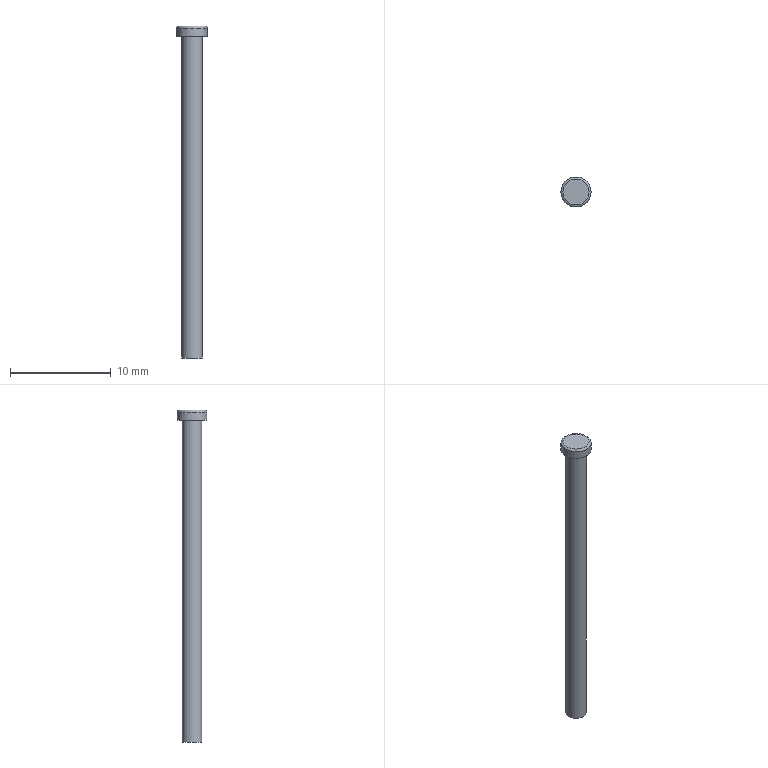Part | STEP file | 1-56.21 | 1 solid | 6 faces | box 3 x 3 x 33 mm | volume 107.521 mm3 | plane 3 | cylinder 2 | torus 1 | commonest cylinder face diameters 2 x1 3 x1
STEP:
#1=CARTESIAN_POINT('',(0.,0.,0.));
#2=DIRECTION('',(0.,0.,1.));
#3=DIRECTION('',(1.,0.,0.));
#4=AXIS2_PLACEMENT_3D('',#1,#2,#3);
#5=CARTESIAN_POINT('',(1.,0.,-32.));
#6=VERTEX_POINT('',#5);
#7=CARTESIAN_POINT('',(0.,0.,-32.));
#8=DIRECTION('',(0.,0.,1.));
#9=DIRECTION('',(1.,0.,0.));
#10=AXIS2_PLACEMENT_3D('',#7,#8,#9);
#11=CIRCLE('',#10,1.);
#12=CARTESIAN_POINT('',(-0.2679,0.,-32.));
#13=DIRECTION('',(0.,0.,1.));
#14=DIRECTION('',(1.,0.,0.));
#15=AXIS2_PLACEMENT_3D('',#12,#13,#14);
#16=PLANE('',#15);
#17=CARTESIAN_POINT('',(0.2679,0.));
#18=DIRECTION('',(1.,0.));
#19=AXIS2_PLACEMENT_2D('',#17,#18);
#20=CIRCLE('',#19,1.);
#21=(GEOMETRIC_REPRESENTATION_CONTEXT(2)PARAMETRIC_REPRESENTATION_CONTEXT()REPRESENTATION_CONTEXT('',''));
#22=DEFINITIONAL_REPRESENTATION('',(#20),#21);
#23=PCURVE('',#16,#22);
#24=CARTESIAN_POINT('',(0.,0.,0.));
#25=DIRECTION('',(0.,0.,-1.));
#26=DIRECTION('',(1.,0.,0.));
#27=AXIS2_PLACEMENT_3D('',#24,#25,#26);
#28=CYLINDRICAL_SURFACE('',#27,1.);
#29=CARTESIAN_POINT('',(6.283,32.));
#30=DIRECTION('',(-1.,0.));
#31=VECTOR('',#30,1.);
#32=LINE('',#29,#31);
#33=(GEOMETRIC_REPRESENTATION_CONTEXT(2)PARAMETRIC_REPRESENTATION_CONTEXT()REPRESENTATION_CONTEXT('',''));
#34=DEFINITIONAL_REPRESENTATION('',(#32),#33);
#35=PCURVE('',#28,#34);
#36=SURFACE_CURVE('',#11,(#23,#35),.PCURVE_S1.);
#37=EDGE_CURVE('',#6,#6,#36,.T.);
#38=ORIENTED_EDGE('',*,*,#37,.T.);
#39=EDGE_LOOP('',(#38));
#40=FACE_BOUND('',#39,.F.);
#41=ADVANCED_FACE('',(#40),#16,.F.);
#42=CARTESIAN_POINT('',(1.,0.,0.));
#43=VERTEX_POINT('',#42);
#44=CARTESIAN_POINT('',(1.,0.,0.));
#45=DIRECTION('',(0.,0.,-1.));
#46=VECTOR('',#45,1.);
#47=LINE('',#44,#46);
#48=CARTESIAN_POINT('',(6.283,0.));
#49=DIRECTION('',(0.,1.));
#50=VECTOR('',#49,1.);
#51=LINE('',#48,#50);
#52=(GEOMETRIC_REPRESENTATION_CONTEXT(2)PARAMETRIC_REPRESENTATION_CONTEXT()REPRESENTATION_CONTEXT('',''));
#53=DEFINITIONAL_REPRESENTATION('',(#51),#52);
#54=PCURVE('',#28,#53);
#55=CARTESIAN_POINT('',(0.,0.));
#56=DIRECTION('',(0.,1.));
#57=VECTOR('',#56,1.);
#58=LINE('',#55,#57);
#59=(GEOMETRIC_REPRESENTATION_CONTEXT(2)PARAMETRIC_REPRESENTATION_CONTEXT()REPRESENTATION_CONTEXT('',''));
#60=DEFINITIONAL_REPRESENTATION('',(#58),#59);
#61=PCURVE('',#28,#60);
#62=SEAM_CURVE('',#47,(#54,#61),.PCURVE_S1.);
#63=EDGE_CURVE('',#43,#6,#62,.T.);
#64=ORIENTED_EDGE('',*,*,#63,.T.);
#65=ORIENTED_EDGE('',*,*,#37,.T.);
#66=ORIENTED_EDGE('',*,*,#63,.F.);
#67=CARTESIAN_POINT('',(0.,0.,0.));
#68=DIRECTION('',(0.,0.,1.));
#69=DIRECTION('',(1.,0.,0.));
#70=AXIS2_PLACEMENT_3D('',#67,#68,#69);
#71=CIRCLE('',#70,1.);
#72=CARTESIAN_POINT('',(6.283,0.));
#73=DIRECTION('',(-1.,0.));
#74=VECTOR('',#73,1.);
#75=LINE('',#72,#74);
#76=(GEOMETRIC_REPRESENTATION_CONTEXT(2)PARAMETRIC_REPRESENTATION_CONTEXT()REPRESENTATION_CONTEXT('',''));
#77=DEFINITIONAL_REPRESENTATION('',(#75),#76);
#78=PCURVE('',#28,#77);
#79=CARTESIAN_POINT('',(-0.4019,0.,0.));
#80=DIRECTION('',(0.,0.,1.));
#81=DIRECTION('',(1.,0.,0.));
#82=AXIS2_PLACEMENT_3D('',#79,#80,#81);
#83=PLANE('',#82);
#84=CARTESIAN_POINT('',(0.4019,0.));
#85=DIRECTION('',(1.,0.));
#86=AXIS2_PLACEMENT_2D('',#84,#85);
#87=CIRCLE('',#86,1.);
#88=(GEOMETRIC_REPRESENTATION_CONTEXT(2)PARAMETRIC_REPRESENTATION_CONTEXT()REPRESENTATION_CONTEXT('',''));
#89=DEFINITIONAL_REPRESENTATION('',(#87),#88);
#90=PCURVE('',#83,#89);
#91=SURFACE_CURVE('',#71,(#78,#90),.PCURVE_S1.);
#92=EDGE_CURVE('',#43,#43,#91,.T.);
#93=ORIENTED_EDGE('',*,*,#92,.F.);
#94=EDGE_LOOP('',(#64,#65,#66,#93));
#95=FACE_BOUND('',#94,.T.);
#96=ADVANCED_FACE('',(#95),#28,.T.);
#97=CARTESIAN_POINT('',(1.5,0.,0.));
#98=VERTEX_POINT('',#97);
#99=CARTESIAN_POINT('',(0.,0.,0.));
#100=DIRECTION('',(0.,0.,1.));
#101=DIRECTION('',(1.,0.,0.));
#102=AXIS2_PLACEMENT_3D('',#99,#100,#101);
#103=CIRCLE('',#102,1.5);
#104=CARTESIAN_POINT('',(0.4019,0.));
#105=DIRECTION('',(1.,0.));
#106=AXIS2_PLACEMENT_2D('',#104,#105);
#107=CIRCLE('',#106,1.5);
#108=(GEOMETRIC_REPRESENTATION_CONTEXT(2)PARAMETRIC_REPRESENTATION_CONTEXT()REPRESENTATION_CONTEXT('',''));
#109=DEFINITIONAL_REPRESENTATION('',(#107),#108);
#110=PCURVE('',#83,#109);
#111=CARTESIAN_POINT('',(0.,0.,0.));
#112=DIRECTION('',(0.,0.,1.));
#113=DIRECTION('',(1.,0.,0.));
#114=AXIS2_PLACEMENT_3D('',#111,#112,#113);
#115=CYLINDRICAL_SURFACE('',#114,1.5);
#116=CARTESIAN_POINT('',(0.,0.));
#117=DIRECTION('',(1.,0.));
#118=VECTOR('',#117,1.);
#119=LINE('',#116,#118);
#120=(GEOMETRIC_REPRESENTATION_CONTEXT(2)PARAMETRIC_REPRESENTATION_CONTEXT()REPRESENTATION_CONTEXT('',''));
#121=DEFINITIONAL_REPRESENTATION('',(#119),#120);
#122=PCURVE('',#115,#121);
#123=SURFACE_CURVE('',#103,(#110,#122),.PCURVE_S1.);
#124=EDGE_CURVE('',#98,#98,#123,.T.);
#125=ORIENTED_EDGE('',*,*,#124,.T.);
#126=EDGE_LOOP('',(#125));
#127=FACE_BOUND('',#126,.F.);
#128=ORIENTED_EDGE('',*,*,#92,.F.);
#129=EDGE_LOOP('',(#128));
#130=FACE_BOUND('',#129,.F.);
#131=ADVANCED_FACE('',(#127,#130),#83,.F.);
#132=ORIENTED_EDGE('',*,*,#124,.T.);
#133=CARTESIAN_POINT('',(1.5,0.,0.8));
#134=VERTEX_POINT('',#133);
#135=CARTESIAN_POINT('',(1.5,0.,0.));
#136=DIRECTION('',(0.,0.,1.));
#137=VECTOR('',#136,1.);
#138=LINE('',#135,#137);
#139=CARTESIAN_POINT('',(6.283,0.));
#140=DIRECTION('',(0.,1.));
#141=VECTOR('',#140,1.);
#142=LINE('',#139,#141);
#143=(GEOMETRIC_REPRESENTATION_CONTEXT(2)PARAMETRIC_REPRESENTATION_CONTEXT()REPRESENTATION_CONTEXT('',''));
#144=DEFINITIONAL_REPRESENTATION('',(#142),#143);
#145=PCURVE('',#115,#144);
#146=CARTESIAN_POINT('',(0.,0.));
#147=DIRECTION('',(0.,1.));
#148=VECTOR('',#147,1.);
#149=LINE('',#146,#148);
#150=(GEOMETRIC_REPRESENTATION_CONTEXT(2)PARAMETRIC_REPRESENTATION_CONTEXT()REPRESENTATION_CONTEXT('',''));
#151=DEFINITIONAL_REPRESENTATION('',(#149),#150);
#152=PCURVE('',#115,#151);
#153=SEAM_CURVE('',#138,(#145,#152),.PCURVE_S1.);
#154=EDGE_CURVE('',#98,#134,#153,.T.);
#155=ORIENTED_EDGE('',*,*,#154,.T.);
#156=CARTESIAN_POINT('',(0.,0.,0.8));
#157=DIRECTION('',(0.,0.,-1.));
#158=DIRECTION('',(1.,0.,0.));
#159=AXIS2_PLACEMENT_3D('',#156,#157,#158);
#160=CIRCLE('',#159,1.5);
#161=CARTESIAN_POINT('',(6.283,0.8));
#162=DIRECTION('',(-1.,0.));
#163=VECTOR('',#162,1.);
#164=LINE('',#161,#163);
#165=(GEOMETRIC_REPRESENTATION_CONTEXT(2)PARAMETRIC_REPRESENTATION_CONTEXT()REPRESENTATION_CONTEXT('',''));
#166=DEFINITIONAL_REPRESENTATION('',(#164),#165);
#167=PCURVE('',#115,#166);
#168=CARTESIAN_POINT('',(0.,0.,0.8));
#169=DIRECTION('',(0.,0.,1.));
#170=DIRECTION('',(1.,0.,0.));
#171=AXIS2_PLACEMENT_3D('',#168,#169,#170);
#172=TOROIDAL_SURFACE('',#171,1.3,0.2);
#173=CARTESIAN_POINT('',(6.283,0.));
#174=DIRECTION('',(-1.,0.));
#175=VECTOR('',#174,1.);
#176=LINE('',#173,#175);
#177=(GEOMETRIC_REPRESENTATION_CONTEXT(2)PARAMETRIC_REPRESENTATION_CONTEXT()REPRESENTATION_CONTEXT('',''));
#178=DEFINITIONAL_REPRESENTATION('',(#176),#177);
#179=PCURVE('',#172,#178);
#180=SURFACE_CURVE('',#160,(#167,#179),.PCURVE_S1.);
#181=EDGE_CURVE('',#134,#134,#180,.T.);
#182=ORIENTED_EDGE('',*,*,#181,.T.);
#183=ORIENTED_EDGE('',*,*,#154,.F.);
#184=EDGE_LOOP('',(#132,#155,#182,#183));
#185=FACE_BOUND('',#184,.T.);
#186=ADVANCED_FACE('',(#185),#115,.T.);
#187=CARTESIAN_POINT('',(1.3,0.,1.));
#188=VERTEX_POINT('',#187);
#189=CARTESIAN_POINT('',(0.,0.,1.));
#190=DIRECTION('',(0.,0.,-1.));
#191=DIRECTION('',(1.,0.,0.));
#192=AXIS2_PLACEMENT_3D('',#189,#190,#191);
#193=CIRCLE('',#192,1.3);
#194=CARTESIAN_POINT('',(-0.4019,0.,1.));
#195=DIRECTION('',(0.,0.,1.));
#196=DIRECTION('',(1.,0.,0.));
#197=AXIS2_PLACEMENT_3D('',#194,#195,#196);
#198=PLANE('',#197);
#199=CARTESIAN_POINT('',(1.702,0.));
#200=CARTESIAN_POINT('',(1.702,-2.252));
#201=CARTESIAN_POINT('',(-0.2481,-1.126));
#202=CARTESIAN_POINT('',(-2.198,0.));
#203=CARTESIAN_POINT('',(-0.2481,1.126));
#204=CARTESIAN_POINT('',(1.702,2.252));
#205=CARTESIAN_POINT('',(1.702,0.));
#206=(BOUNDED_CURVE()B_SPLINE_CURVE(2,(#199,#200,#201,#202,#203,#204,#205),.UNSPECIFIED.,.T.,.F.)B_SPLINE_CURVE_WITH_KNOTS((1,2,2,2,2,1),(-2.094,0.,2.094,4.189,6.283,8.378),.UNSPECIFIED.)CURVE()GEOMETRIC_REPRESENTATION_ITEM()RATIONAL_B_SPLINE_CURVE((1.,0.5,1.,0.5,1.,0.5,1.))REPRESENTATION_ITEM(''));
#207=(GEOMETRIC_REPRESENTATION_CONTEXT(2)PARAMETRIC_REPRESENTATION_CONTEXT()REPRESENTATION_CONTEXT('',''));
#208=DEFINITIONAL_REPRESENTATION('',(#206),#207);
#209=PCURVE('',#198,#208);
#210=CARTESIAN_POINT('',(6.283,1.571));
#211=DIRECTION('',(-1.,0.));
#212=VECTOR('',#211,1.);
#213=LINE('',#210,#212);
#214=(GEOMETRIC_REPRESENTATION_CONTEXT(2)PARAMETRIC_REPRESENTATION_CONTEXT()REPRESENTATION_CONTEXT('',''));
#215=DEFINITIONAL_REPRESENTATION('',(#213),#214);
#216=PCURVE('',#172,#215);
#217=SURFACE_CURVE('',#193,(#209,#216),.PCURVE_S1.);
#218=EDGE_CURVE('',#188,#188,#217,.T.);
#219=ORIENTED_EDGE('',*,*,#218,.F.);
#220=EDGE_LOOP('',(#219));
#221=FACE_BOUND('',#220,.T.);
#222=ADVANCED_FACE('',(#221),#198,.T.);
#223=CARTESIAN_POINT('',(1.3,0.,0.8));
#224=DIRECTION('',(0.,1.,0.));
#225=DIRECTION('',(0.,0.,1.));
#226=AXIS2_PLACEMENT_3D('',#223,#224,#225);
#227=CIRCLE('',#226,0.2);
#228=CARTESIAN_POINT('',(0.,1.571));
#229=DIRECTION('',(0.,-1.));
#230=VECTOR('',#229,1.);
#231=LINE('',#228,#230);
#232=(GEOMETRIC_REPRESENTATION_CONTEXT(2)PARAMETRIC_REPRESENTATION_CONTEXT()REPRESENTATION_CONTEXT('',''));
#233=DEFINITIONAL_REPRESENTATION('',(#231),#232);
#234=PCURVE('',#172,#233);
#235=CARTESIAN_POINT('',(6.283,1.571));
#236=DIRECTION('',(0.,-1.));
#237=VECTOR('',#236,1.);
#238=LINE('',#235,#237);
#239=(GEOMETRIC_REPRESENTATION_CONTEXT(2)PARAMETRIC_REPRESENTATION_CONTEXT()REPRESENTATION_CONTEXT('',''));
#240=DEFINITIONAL_REPRESENTATION('',(#238),#239);
#241=PCURVE('',#172,#240);
#242=SEAM_CURVE('',#227,(#234,#241),.PCURVE_S1.);
#243=EDGE_CURVE('',#188,#134,#242,.T.);
#244=ORIENTED_EDGE('',*,*,#243,.T.);
#245=ORIENTED_EDGE('',*,*,#181,.F.);
#246=ORIENTED_EDGE('',*,*,#243,.F.);
#247=ORIENTED_EDGE('',*,*,#218,.T.);
#248=EDGE_LOOP('',(#244,#245,#246,#247));
#249=FACE_BOUND('',#248,.T.);
#250=ADVANCED_FACE('',(#249),#172,.T.);
#251=CLOSED_SHELL('',(#41,#96,#131,#186,#222,#250));
#252=MANIFOLD_SOLID_BREP('',#251);
#253=(LENGTH_UNIT()NAMED_UNIT(*)SI_UNIT(.MILLI.,.METRE.));
#254=UNCERTAINTY_MEASURE_WITH_UNIT(LENGTH_MEASURE(0.0000001),#253,'','');
#255=(NAMED_UNIT(*)PLANE_ANGLE_UNIT()SI_UNIT($,.RADIAN.));
#256=(NAMED_UNIT(*)SI_UNIT($,.STERADIAN.)SOLID_ANGLE_UNIT());
#257=(GEOMETRIC_REPRESENTATION_CONTEXT(3)GLOBAL_UNCERTAINTY_ASSIGNED_CONTEXT((#254))GLOBAL_UNIT_ASSIGNED_CONTEXT((#253,#255,#256))REPRESENTATION_CONTEXT('',''));
#258=ADVANCED_BREP_SHAPE_REPRESENTATION('',(#4,#252),#257);